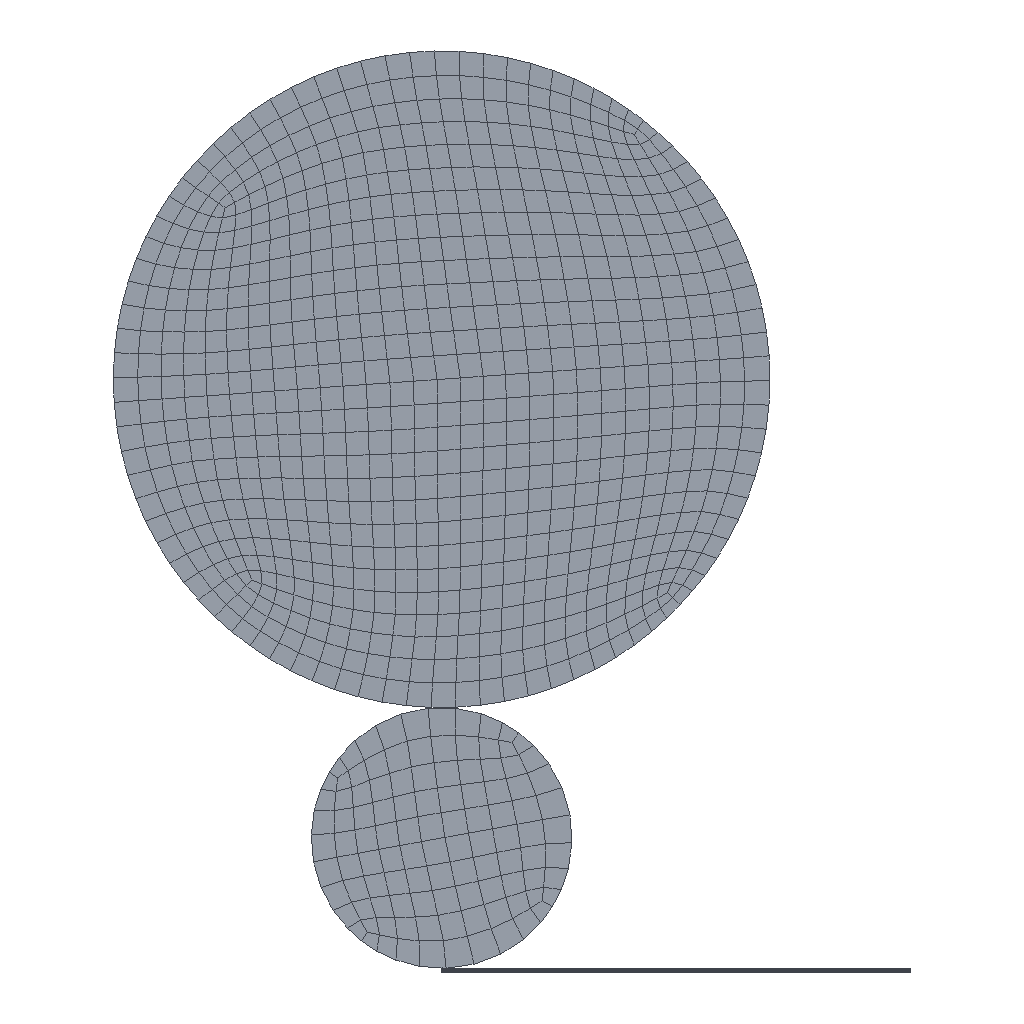Simulation study | abaqus
Set-up summary:
category,name,step,type,value,unit,region
solver,abaqus,,Abaqus/CAE 2024
units,mm-N-s-tonne (MPa),,inferred,E=210000 density=8.2e-09
analysis,JIECHU,,dynamic explicit,nlgeom=True; time_period=0.1
analysis,YAXIA,,dynamic explicit,nlgeom=True; time_period=0.1
mesh,nodes,,,3921
mesh,elements,,,3350
element_type,CPE4RT,,,3350
material,hss,,E,210000
material,hss,,nu,0.3
material,hss,,density,8.2e-09
material,hss,,conductivity,27
material,hss,,specific_heat,460000
material,hss,,cte,1.16e-05
material,hss,,behaviors,conductivity; expansion; specific heat
material,q235,,E,190000
material,q235,,nu,0.3
material,q235,,density,7.85e-09
material,q235,,yield,104.87
material,q235,,conductivity,47
material,q235,,specific_heat,470000
material,q235,,cte,1.2e-05
material,q235,,behaviors,plastic; conductivity; expansion; rate dependent; specific heat
section,q235,,solid section,,,Q235
section,hss,,solid section,,,GZG
section,hss,,solid section,,,ZCG
load,ban-wendu,initial,initial condition temperature
load,gzg-wendu,initial,initial condition temperature
load,zcg-wendu,initial,initial condition temperature
bc,duichenban,initial,ysymm,[dofs=YSYMM],,ban-1.Q235
bc,BAN-JIECHU,JIECHU,fixed,"[dofs=rz,x,y n=3]",,YUAN-BAN
bc,GZG-JIECHU,JIECHU,fixed,"[dofs=rz,x n=2]",,m_Set-1
bc,zcg-jiechu,JIECHU,fixed,"[dofs=rz,x n=2]",,m_Set-2
bc,zcg-jiechu,JIECHU,displacement,-0.01 [dofs=y],,m_Set-2
bc,BAN-YAXIA,YAXIA,fixed,"[dofs=rz,y n=2]",,YUAN-BAN
bc,zcg-yaxia,YAXIA,fixed,"[dofs=rz,x n=2]",,m_Set-2
bc,zcg-yaxia,YAXIA,displacement,-3.5 [dofs=y],,m_Set-2
contact,Int-4,initial,general contact,interaction=IntProp-1; friction=0.2; behavior=hard
constraint,coupling,,,2
Abaqus input file, long lists of numbers shortened:
*Heading
** Job name: deck Model name: Model-1
** Generated by: Abaqus/CAE 2024
*Preprint, echo=NO, model=NO, history=NO, contact=NO
**
** PARTS
**
*Part, name=ban
*Node
      1,        1000.,        -3.75
      2,         998.,        -3.75
** (3004 more lines like these left out)
*Element, type=CPE4RT
   1,    1,    2,  503,  502
   2,    2,    3,  504,  503
** (2498 more lines like these left out)
*Nset, nset=Q235, generate
    1,  3006,     1
*Elset, elset=Q235, generate
    1,  2500,     1
** Section: Q235
*Solid Section, elset=Q235, material=q235
,
*End Part
**
*Part, name=gzg
*Node
      1,   9.599,  -277.834
      2,  -43.246,  -7.894
** (122 more lines like these left out)
*Element, type=CPE4RT
  1,   9,  10,  56,  53
  2,  10,  11,  55,  56
** (104 more lines like these left out)
*Nset, nset=GZG, generate
   1,  124,    1
*Elset, elset=GZG, generate
   1,  106,    1
** Section: HSS
*Solid Section, elset=GZG, material=hss
,
*End Part
**
*Part, name=zcg
*Node
      1,   37.004,    699.021
      2,   136.114,   9.72
** (787 more lines like these left out)
*Element, type=CPE4RT
  1,  17,  18, 163, 151
  2,  18,  19, 164, 163
** (742 more lines like these left out)
*Nset, nset=ZCG, generate
   1,  789,    1
*Elset, elset=ZCG, generate
   1,  744,    1
** Section: HSS
*Solid Section, elset=ZCG, material=hss
,
*End Part
**
**
** ASSEMBLY
**
*Assembly, name=Assembly
**
*Instance, name=gzg-1, part=gzg
          0.,         288.,           0.
*End Instance
**
*Instance, name=zcg-1, part=zcg
          0.,        1266.,           0.
*End Instance
**
*Instance, name=ban-1, part=ban
          0.,        13.75,           0.
*End Instance
**
*Node
      1,           0.,         288.,           0.
*Node
      2,           0.,        1266.,           0.
*Nset, nset=YUAN-BAN, instance=ban-1, generate
    1,  2506,   501
*Elset, elset=YUAN-BAN, instance=ban-1, generate
    1,  2001,   500
*Nset, nset=m_Set-1
 1,
*Nset, nset=m_Set-2
 2,
*Elset, elset=_BAN-SURF_S1, internal, instance=ban-1, generate
   1,  500,    1
*Elset, elset=_BAN-SURF_S2, internal, instance=ban-1, generate
  500,  2500,   500
*Surface, type=ELEMENT, name=BAN-SURF
_BAN-SURF_S1, S1
_BAN-SURF_S2, S2
*Elset, elset=_m_Surf-1_S1, internal, instance=gzg-1
  1,  2,  3,  4, 50, 51, 52, 53, 74, 75, 76, 77, 78, 79, 80, 81
 82,
*Elset, elset=_m_Surf-1_S2, internal, instance=gzg-1
  21,  22,  23,  24,  45,  46,  47,  48,  49,  70,  71,  72,  73, 103, 104, 105
 106,
*Surface, type=ELEMENT, name=m_Surf-1
_m_Surf-1_S1, S1
_m_Surf-1_S2, S2
*Elset, elset=_s_Surf-1_S1, internal, instance=zcg-1
   1,   2,   3,   4,   5,   6,   7,   8,   9, 333, 334, 335, 336, 337, 338, 339
 340, 341, 342, 499, 500, 501, 502, 503, 504, 505, 506, 507, 508, 509, 510, 523
** (1 more lines like these left out)
*Elset, elset=_s_Surf-1_S2, internal, instance=zcg-1
 128, 130, 132, 134, 136, 138, 140, 142, 144, 146, 148, 150, 284, 288, 292, 296
 300, 304, 308, 312, 316, 320, 324, 328, 332, 482, 484, 486, 488, 490, 492, 494
** (1 more lines like these left out)
*Surface, type=ELEMENT, name=s_Surf-1
_s_Surf-1_S1, S1
_s_Surf-1_S2, S2
** Constraint: OUHE1
*Coupling, constraint name=OUHE1, ref node=m_Set-1, surface=m_Surf-1
*Kinematic
** Constraint: OUHE2
*Coupling, constraint name=OUHE2, ref node=m_Set-2, surface=s_Surf-1
*Kinematic
*End Assembly
*Amplitude, name=Amp-1
             0.,              0.,            0.01,              1.
*Amplitude, name=Amp-2
             0.,              0.,            0.01,              1.
*Amplitude, name=Amp-4
             0.,              0.,           0.001,              1.
**
** MATERIALS
**
*Material, name=hss
*Conductivity
27.,
*Density
 8.2e-09,
*Elastic
210000., 0.3
*Expansion
 1.16e-05,
*Specific Heat
460000.,
*Material, name=q235
*Conductivity
47.,
*Density
 7.85e-09,
*Elastic
190000., 0.3
*Expansion
 1.2e-05,
*Plastic, hardening=JOHNSON COOK
 104.87,  178.63, 0.2564, 0.682,   1773.,    298.
*Rate Dependent, type=JOHNSON COOK
 0.08139, 0.05
*Specific Heat
470000.,
**
** INTERACTION PROPERTIES
**
*Surface Interaction, name=IntProp-1
*Friction
 0.2,
*Surface Behavior, pressure-overclosure=HARD
*Gap Conductance
1000., 0.
   0.,10.
*Gap Heat Generation
1., 0.5
*Surface Interaction, name=IntProp-2
*Friction
 0.6,
*Surface Behavior, pressure-overclosure=HARD
*Gap Conductance
5000., 0.
   0.,10.
*Gap Heat Generation
1., 0.5
**
** BOUNDARY CONDITIONS
**
** Name: duichenban Type: Symmetry/Antisymmetry/Encastre
*Boundary
ban-1.Q235, YSYMM
**
** PREDEFINED FIELDS
**
** Name: ban-wendu   Type: Temperature
*Initial Conditions, type=TEMPERATURE
ban-1.Q235, 1300.
** Name: gzg-wendu   Type: Temperature
*Initial Conditions, type=TEMPERATURE
gzg-1.GZG, 300.
** Name: zcg-wendu   Type: Temperature
*Initial Conditions, type=TEMPERATURE
zcg-1.ZCG, 300.
**
** INTERACTIONS
**
** Interaction: Int-4
*Contact, op=NEW
*Contact Inclusions, ALL EXTERIOR
*Contact Property Assignment
 ,  , IntProp-1
** ----------------------------------------------------------------
**
** STEP: JIECHU
**
*Step, name=JIECHU, nlgeom=YES
*Dynamic, Explicit
, 0.1
*Bulk Viscosity
0.06, 1.2
** Mass Scaling: Semi-Automatic
**               Whole Model
*Fixed Mass Scaling, factor=100.
**
** BOUNDARY CONDITIONS
**
** Name: BAN-JIECHU Type: Displacement/Rotation
*Boundary
YUAN-BAN, 1, 1
YUAN-BAN, 2, 2
YUAN-BAN, 6, 6
** Name: GZG-JIECHU Type: Displacement/Rotation
*Boundary
m_Set-1, 1, 1
m_Set-1, 6, 6
** Name: zcg-jiechu Type: Displacement/Rotation
*Boundary, amplitude=Amp-1
m_Set-2, 1, 1
m_Set-2, 2, 2, -0.01
m_Set-2, 6, 6
**
** OUTPUT REQUESTS
**
*Restart, write, number interval=1, time marks=NO
**
** FIELD OUTPUT: F-Output-1
**
*Output, field, variable=PRESELECT
**
** HISTORY OUTPUT: H-Output-1
**
*Output, history, variable=PRESELECT
*End Step
** ----------------------------------------------------------------
**
** STEP: YAXIA
**
*Step, name=YAXIA, nlgeom=YES
*Dynamic, Explicit
, 0.1
*Bulk Viscosity
0.06, 1.2
** Mass Scaling: Semi-Automatic
**               Whole Model
*Fixed Mass Scaling, factor=100.
**
** BOUNDARY CONDITIONS
**
** Name: BAN-YAXIA Type: Displacement/Rotation
*Boundary
YUAN-BAN, 2, 2
YUAN-BAN, 6, 6
** Name: zcg-yaxia Type: Displacement/Rotation
*Boundary, amplitude=Amp-4
m_Set-2, 1, 1
m_Set-2, 2, 2, -3.5
m_Set-2, 6, 6
**
** OUTPUT REQUESTS
**
*Restart, write, number interval=1, time marks=NO
**
** FIELD OUTPUT: F-Output-1
**
*Output, field, variable=PRESELECT
**
** HISTORY OUTPUT: H-Output-1
**
*Output, history, variable=PRESELECT
*End Step
Results summary:
result,odb.job_status,,,JOB_STATUS_COMPLETED_SUCCESSFULLY,"consistent, unstated (Abaqus has no unit system)"
result,steps[0].procedure,JIECHU,,"*DYNAMIC, EXPLICIT","consistent, unstated (Abaqus has no unit system)"
result,steps[0].time_period,JIECHU,,0.1,"consistent, unstated (Abaqus has no unit system)"
result,steps[0].n_frames,JIECHU,,21,"consistent, unstated (Abaqus has no unit system)"
result,steps[0].last_frame.id,JIECHU,,33230,"consistent, unstated (Abaqus has no unit system)"
result,steps[0].last_frame.value,JIECHU,,0.1,"consistent, unstated (Abaqus has no unit system)"
result,steps[0].last_frame.description,JIECHU,,Increment     33230: Step Time =   0.1,"consistent, unstated (Abaqus has no unit system)"
result,steps[0].completed,JIECHU,,True,"consistent, unstated (Abaqus has no unit system)"
result,steps[0].max_U_magnitude,JIECHU,,0.01,"consistent, unstated (Abaqus has no unit system)"
result,steps[0].max_S_mises,JIECHU,,0.4798,"consistent, unstated (Abaqus has no unit system)"
result,steps[0].RF_sum[1],JIECHU,,1.492,"consistent, unstated (Abaqus has no unit system)"
result,steps[0].RF_sum[2],JIECHU,,-2020.65,"consistent, unstated (Abaqus has no unit system)"
result,steps[0].diagnostic.n_increments,JIECHU,,21,"consistent, unstated (Abaqus has no unit system)"
result,steps[1].procedure,YAXIA,,"*DYNAMIC, EXPLICIT","consistent, unstated (Abaqus has no unit system)"
result,steps[1].time_period,YAXIA,,0.1,"consistent, unstated (Abaqus has no unit system)"
result,steps[1].n_frames,YAXIA,,21,"consistent, unstated (Abaqus has no unit system)"
result,steps[1].last_frame.id,YAXIA,,34120,"consistent, unstated (Abaqus has no unit system)"
result,steps[1].last_frame.value,YAXIA,,0.1,"consistent, unstated (Abaqus has no unit system)"
result,steps[1].last_frame.description,YAXIA,,Increment     34120: Step Time =   0.1,"consistent, unstated (Abaqus has no unit system)"
result,steps[1].completed,YAXIA,,True,"consistent, unstated (Abaqus has no unit system)"
result,steps[1].max_U_magnitude,YAXIA,,3.883,"consistent, unstated (Abaqus has no unit system)"
result,steps[1].max_S_mises,YAXIA,,1410.47,"consistent, unstated (Abaqus has no unit system)"
result,steps[1].RF_sum[1],YAXIA,,-36304.9,"consistent, unstated (Abaqus has no unit system)"
result,steps[1].RF_sum[2],YAXIA,,-2.32631e+06,"consistent, unstated (Abaqus has no unit system)"
result,steps[1].diagnostic.n_increments,YAXIA,,21,"consistent, unstated (Abaqus has no unit system)"